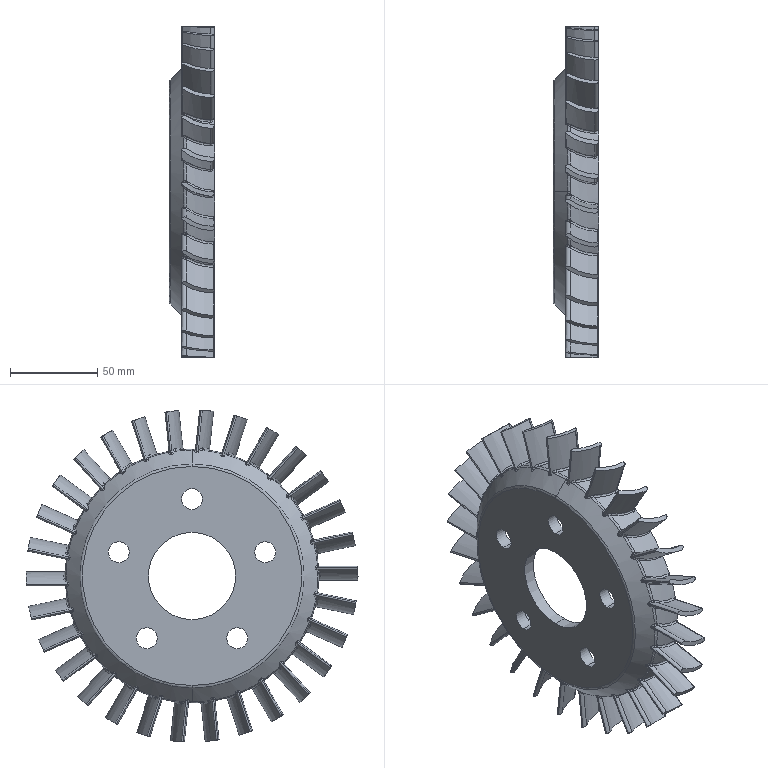Part | STEP file | Previa 01.sldasm-Part-4_Valor predeterminado | 1 solid | 685 faces | box 26.228 x 190 x 189.8 mm | volume 157872 mm3 | spline 360 | cylinder 285 | torus 33 | cone 4 | plane 3 | commonest cylinder face diameters 4 x90 1.2 x60 145 x31 53.531 x30 58.531 x30 190 x30